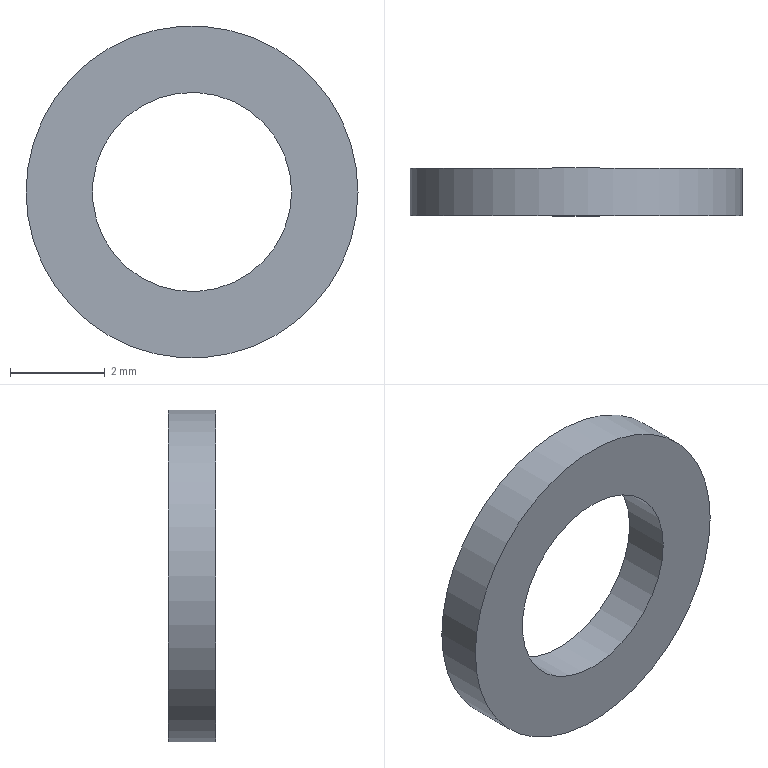Part | NX | features DATUM_CSYS 2, EXTRUDE 1, SKETCH 1 | 1 solid | 4 faces | box 7 x 1 x 7 mm | volume 24.63 mm3 | cylinder 2 | plane 2 | commonest cylinder face diameters 4.2 x1 7 x1
STEP:
#1=CARTESIAN_POINT('',(3.5,-1.,0.));
#2=VERTEX_POINT('',#1);
#3=CARTESIAN_POINT('',(0.,-1.,0.));
#4=DIRECTION('',(0.,1.,0.));
#5=DIRECTION('',(1.,0.,0.));
#6=AXIS2_PLACEMENT_3D('',#3,#4,#5);
#7=CIRCLE('',#6,3.5);
#8=EDGE_CURVE('',#2,#2,#7,.T.);
#9=ORIENTED_EDGE('',*,*,#8,.T.);
#10=EDGE_LOOP('',(#9));
#11=FACE_BOUND('',#10,.T.);
#12=CARTESIAN_POINT('',(3.5,0.,0.));
#13=VERTEX_POINT('',#12);
#14=CARTESIAN_POINT('',(0.,0.,0.));
#15=DIRECTION('',(0.,1.,0.));
#16=DIRECTION('',(1.,0.,0.));
#17=AXIS2_PLACEMENT_3D('',#14,#15,#16);
#18=CIRCLE('',#17,3.5);
#19=EDGE_CURVE('',#13,#13,#18,.T.);
#20=ORIENTED_EDGE('',*,*,#19,.F.);
#21=EDGE_LOOP('',(#20));
#22=FACE_BOUND('',#21,.T.);
#23=CARTESIAN_POINT('',(0.,-1.,0.));
#24=DIRECTION('',(0.,1.,0.));
#25=DIRECTION('',(0.,0.,1.));
#26=AXIS2_PLACEMENT_3D('',#23,#24,#25);
#27=CYLINDRICAL_SURFACE('',#26,3.5);
#28=ADVANCED_FACE('',(#11,#22),#27,.T.);
#29=CARTESIAN_POINT('',(2.1,-1.,0.));
#30=VERTEX_POINT('',#29);
#31=CARTESIAN_POINT('',(0.,-1.,0.));
#32=DIRECTION('',(0.,-1.,0.));
#33=DIRECTION('',(1.,0.,0.));
#34=AXIS2_PLACEMENT_3D('',#31,#32,#33);
#35=CIRCLE('',#34,2.1);
#36=EDGE_CURVE('',#30,#30,#35,.T.);
#37=ORIENTED_EDGE('',*,*,#36,.T.);
#38=EDGE_LOOP('',(#37));
#39=FACE_BOUND('',#38,.T.);
#40=CARTESIAN_POINT('',(2.1,0.,0.));
#41=VERTEX_POINT('',#40);
#42=CARTESIAN_POINT('',(0.,0.,0.));
#43=DIRECTION('',(0.,-1.,0.));
#44=DIRECTION('',(1.,0.,0.));
#45=AXIS2_PLACEMENT_3D('',#42,#43,#44);
#46=CIRCLE('',#45,2.1);
#47=EDGE_CURVE('',#41,#41,#46,.T.);
#48=ORIENTED_EDGE('',*,*,#47,.F.);
#49=EDGE_LOOP('',(#48));
#50=FACE_BOUND('',#49,.T.);
#51=CARTESIAN_POINT('',(0.,-1.,0.));
#52=DIRECTION('',(0.,1.,0.));
#53=DIRECTION('',(0.,0.,1.));
#54=AXIS2_PLACEMENT_3D('',#51,#52,#53);
#55=CYLINDRICAL_SURFACE('',#54,2.1);
#56=ADVANCED_FACE('',(#39,#50),#55,.F.);
#57=ORIENTED_EDGE('',*,*,#8,.F.);
#58=EDGE_LOOP('',(#57));
#59=FACE_BOUND('',#58,.T.);
#60=ORIENTED_EDGE('',*,*,#36,.F.);
#61=EDGE_LOOP('',(#60));
#62=FACE_BOUND('',#61,.T.);
#63=CARTESIAN_POINT('',(0.,-1.,0.));
#64=DIRECTION('',(0.,1.,0.));
#65=DIRECTION('',(0.,0.,1.));
#66=AXIS2_PLACEMENT_3D('',#63,#64,#65);
#67=PLANE('',#66);
#68=ADVANCED_FACE('',(#59,#62),#67,.F.);
#69=ORIENTED_EDGE('',*,*,#19,.T.);
#70=EDGE_LOOP('',(#69));
#71=FACE_BOUND('',#70,.T.);
#72=ORIENTED_EDGE('',*,*,#47,.T.);
#73=EDGE_LOOP('',(#72));
#74=FACE_BOUND('',#73,.T.);
#75=CARTESIAN_POINT('',(0.,0.,0.));
#76=DIRECTION('',(0.,1.,0.));
#77=DIRECTION('',(0.,0.,1.));
#78=AXIS2_PLACEMENT_3D('',#75,#76,#77);
#79=PLANE('',#78);
#80=ADVANCED_FACE('',(#71,#74),#79,.T.);
#81=CLOSED_SHELL('',(#28,#56,#68,#80));
#82=MANIFOLD_SOLID_BREP('',#81);
#83=(LENGTH_UNIT()NAMED_UNIT(*)SI_UNIT(.MILLI.,.METRE.));
#84=UNCERTAINTY_MEASURE_WITH_UNIT(LENGTH_MEASURE(0.00001),#83,'','');
#85=(NAMED_UNIT(*)PLANE_ANGLE_UNIT()SI_UNIT($,.RADIAN.));
#86=(NAMED_UNIT(*)SI_UNIT($,.STERADIAN.)SOLID_ANGLE_UNIT());
#87=(GEOMETRIC_REPRESENTATION_CONTEXT(3)GLOBAL_UNCERTAINTY_ASSIGNED_CONTEXT((#84))GLOBAL_UNIT_ASSIGNED_CONTEXT((#83,#85,#86))REPRESENTATION_CONTEXT('',''));
#88=ADVANCED_BREP_SHAPE_REPRESENTATION('',(#82),#87);